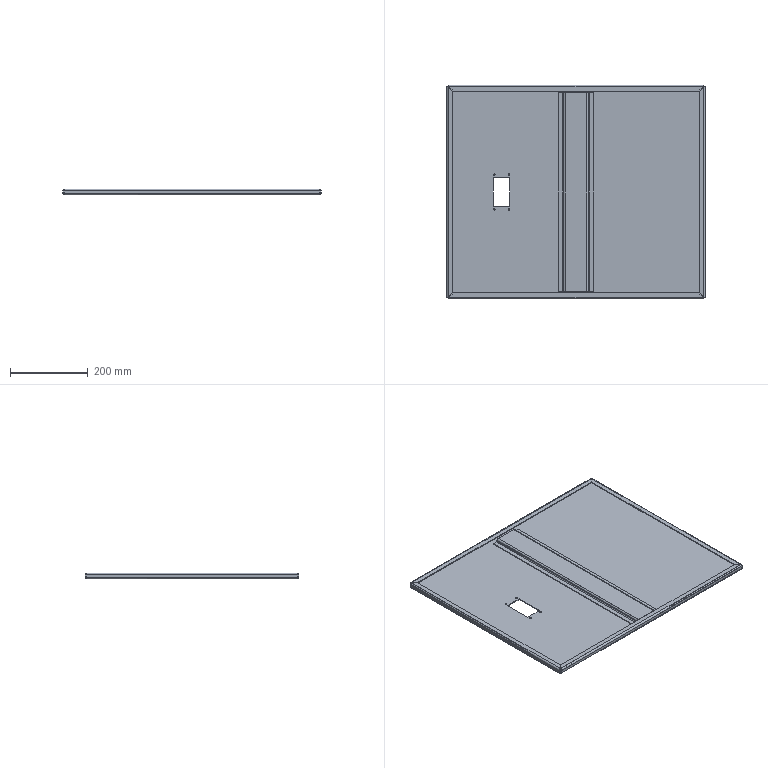Part | SolidWorks | features BaseBody 2 | 2 solids | 104 faces | box 662 x 548 x 15 mm | volume 933031 mm3 | plane 56 | cylinder 32 | spline 16 | commonest cylinder face diameters 4 x12 8 x12 4.5 x8